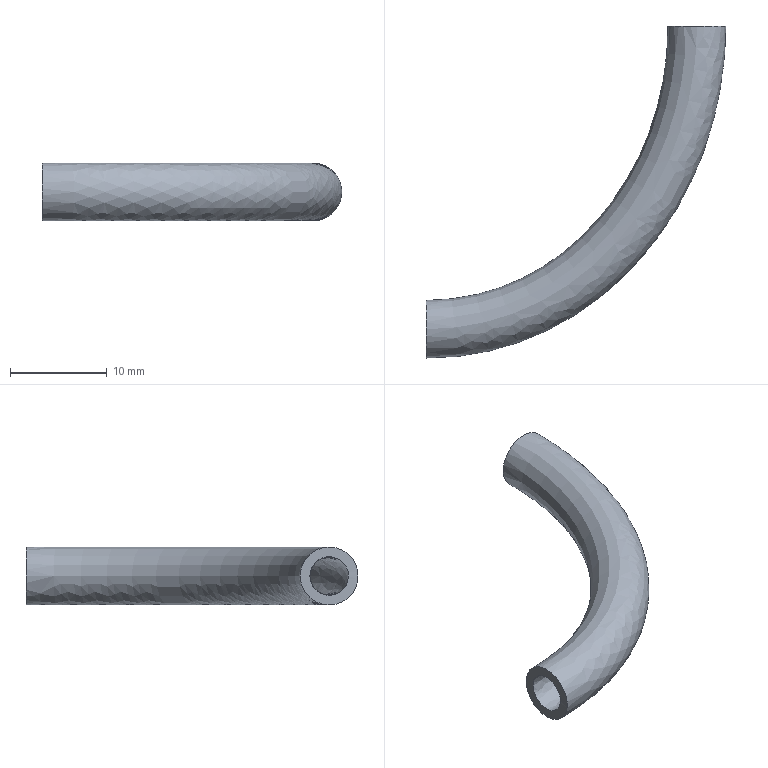Part | NX | features solid 2 | 1 solid | 4 faces | box 31.01 x 34.387 x 6 mm | volume 729.209 mm3 | plane 2 | spline 2